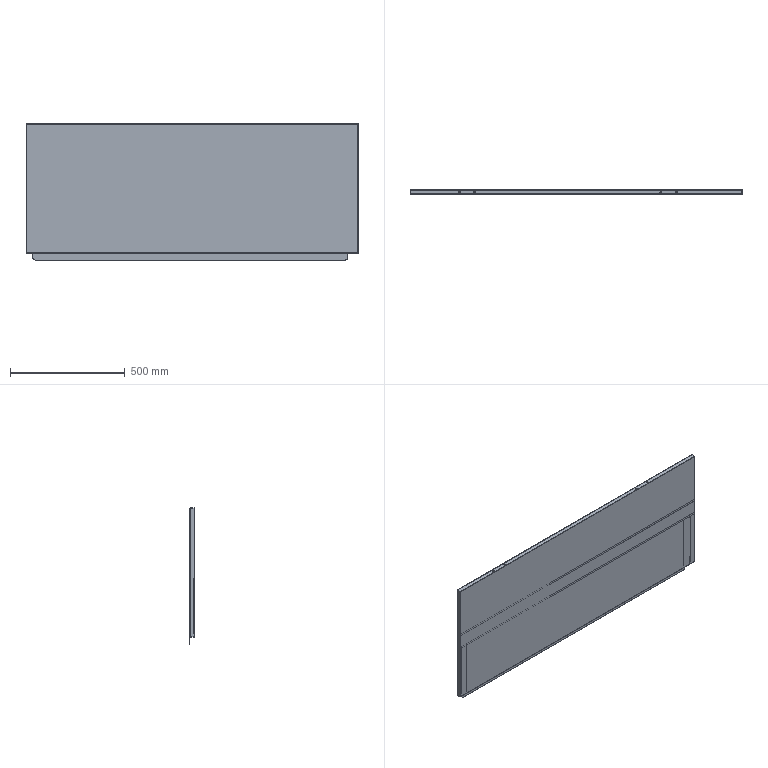Part | SolidWorks | 4 solids | 266 faces | box 1445 x 21.5 x 592 mm | volume 1713091 mm3 | plane 178 | cylinder 84 | spline 4 | commonest cylinder face diameters 3.3 x24 0.4 x20 3.4 x20 3.2 x8 8 x8 0.75 x2